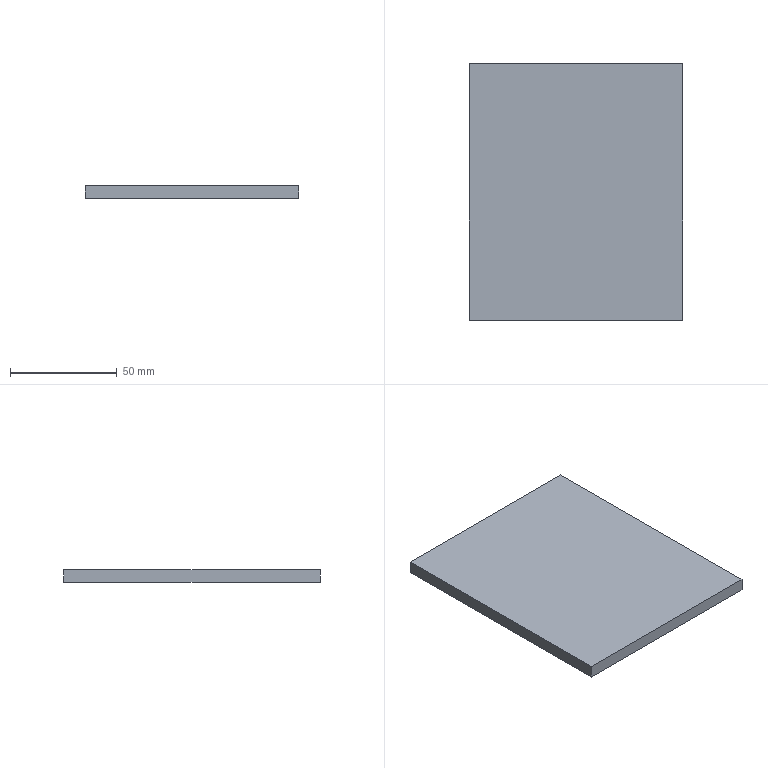Part | SolidWorks | features Extrusion 1 | 1 solid | 6 faces | box 100 x 120 x 6 mm | volume 72000 mm3 | plane 6
STEP:
#1=CARTESIAN_POINT('',(0.,0.,0.));
#2=VERTEX_POINT('',#1);
#3=CARTESIAN_POINT('',(100.,0.,0.));
#4=VERTEX_POINT('',#3);
#5=CARTESIAN_POINT('',(100.,0.,0.));
#6=DIRECTION('',(1.,0.,0.));
#7=VECTOR('',#6,1000.);
#8=LINE('',#5,#7);
#9=EDGE_CURVE('',#2,#4,#8,.T.);
#10=ORIENTED_EDGE('',*,*,#9,.T.);
#11=CARTESIAN_POINT('',(100.,0.,6.));
#12=VERTEX_POINT('',#11);
#13=CARTESIAN_POINT('',(100.,0.,6.));
#14=DIRECTION('',(0.,0.,-1.));
#15=VECTOR('',#14,1000.);
#16=LINE('',#13,#15);
#17=EDGE_CURVE('',#12,#4,#16,.T.);
#18=ORIENTED_EDGE('',*,*,#17,.F.);
#19=CARTESIAN_POINT('',(0.,0.,6.));
#20=VERTEX_POINT('',#19);
#21=CARTESIAN_POINT('',(100.,0.,6.));
#22=DIRECTION('',(1.,0.,0.));
#23=VECTOR('',#22,1000.);
#24=LINE('',#21,#23);
#25=EDGE_CURVE('',#20,#12,#24,.T.);
#26=ORIENTED_EDGE('',*,*,#25,.F.);
#27=CARTESIAN_POINT('',(0.,0.,6.));
#28=DIRECTION('',(0.,0.,-1.));
#29=VECTOR('',#28,1000.);
#30=LINE('',#27,#29);
#31=EDGE_CURVE('',#20,#2,#30,.T.);
#32=ORIENTED_EDGE('',*,*,#31,.T.);
#33=EDGE_LOOP('',(#10,#18,#26,#32));
#34=FACE_OUTER_BOUND('',#33,.T.);
#35=CARTESIAN_POINT('',(100.,0.,6.));
#36=DIRECTION('',(0.,1.,0.));
#37=DIRECTION('',(0.,0.,1.));
#38=AXIS2_PLACEMENT_3D('',#35,#36,#37);
#39=PLANE('',#38);
#40=ADVANCED_FACE('',(#34),#39,.F.);
#41=CARTESIAN_POINT('',(100.,120.,0.));
#42=VERTEX_POINT('',#41);
#43=CARTESIAN_POINT('',(100.,120.,0.));
#44=DIRECTION('',(0.,1.,0.));
#45=VECTOR('',#44,1000.);
#46=LINE('',#43,#45);
#47=EDGE_CURVE('',#4,#42,#46,.T.);
#48=ORIENTED_EDGE('',*,*,#47,.T.);
#49=CARTESIAN_POINT('',(100.,120.,6.));
#50=VERTEX_POINT('',#49);
#51=CARTESIAN_POINT('',(100.,120.,6.));
#52=DIRECTION('',(0.,0.,-1.));
#53=VECTOR('',#52,1000.);
#54=LINE('',#51,#53);
#55=EDGE_CURVE('',#50,#42,#54,.T.);
#56=ORIENTED_EDGE('',*,*,#55,.F.);
#57=CARTESIAN_POINT('',(100.,120.,6.));
#58=DIRECTION('',(0.,1.,0.));
#59=VECTOR('',#58,1000.);
#60=LINE('',#57,#59);
#61=EDGE_CURVE('',#12,#50,#60,.T.);
#62=ORIENTED_EDGE('',*,*,#61,.F.);
#63=ORIENTED_EDGE('',*,*,#17,.T.);
#64=EDGE_LOOP('',(#48,#56,#62,#63));
#65=FACE_OUTER_BOUND('',#64,.T.);
#66=CARTESIAN_POINT('',(100.,120.,6.));
#67=DIRECTION('',(-1.,0.,0.));
#68=DIRECTION('',(0.,0.,1.));
#69=AXIS2_PLACEMENT_3D('',#66,#67,#68);
#70=PLANE('',#69);
#71=ADVANCED_FACE('',(#65),#70,.F.);
#72=CARTESIAN_POINT('',(0.,120.,0.));
#73=VERTEX_POINT('',#72);
#74=CARTESIAN_POINT('',(0.,120.,0.));
#75=DIRECTION('',(-1.,0.,0.));
#76=VECTOR('',#75,1000.);
#77=LINE('',#74,#76);
#78=EDGE_CURVE('',#42,#73,#77,.T.);
#79=ORIENTED_EDGE('',*,*,#78,.T.);
#80=CARTESIAN_POINT('',(0.,120.,6.));
#81=VERTEX_POINT('',#80);
#82=CARTESIAN_POINT('',(0.,120.,6.));
#83=DIRECTION('',(0.,0.,-1.));
#84=VECTOR('',#83,1000.);
#85=LINE('',#82,#84);
#86=EDGE_CURVE('',#81,#73,#85,.T.);
#87=ORIENTED_EDGE('',*,*,#86,.F.);
#88=CARTESIAN_POINT('',(0.,120.,6.));
#89=DIRECTION('',(-1.,0.,0.));
#90=VECTOR('',#89,1000.);
#91=LINE('',#88,#90);
#92=EDGE_CURVE('',#50,#81,#91,.T.);
#93=ORIENTED_EDGE('',*,*,#92,.F.);
#94=ORIENTED_EDGE('',*,*,#55,.T.);
#95=EDGE_LOOP('',(#79,#87,#93,#94));
#96=FACE_OUTER_BOUND('',#95,.T.);
#97=CARTESIAN_POINT('',(0.,120.,6.));
#98=DIRECTION('',(0.,-1.,0.));
#99=DIRECTION('',(0.,0.,-1.));
#100=AXIS2_PLACEMENT_3D('',#97,#98,#99);
#101=PLANE('',#100);
#102=ADVANCED_FACE('',(#96),#101,.F.);
#103=CARTESIAN_POINT('',(0.,0.,0.));
#104=DIRECTION('',(0.,-1.,0.));
#105=VECTOR('',#104,1000.);
#106=LINE('',#103,#105);
#107=EDGE_CURVE('',#73,#2,#106,.T.);
#108=ORIENTED_EDGE('',*,*,#107,.T.);
#109=ORIENTED_EDGE('',*,*,#31,.F.);
#110=CARTESIAN_POINT('',(0.,0.,6.));
#111=DIRECTION('',(0.,-1.,0.));
#112=VECTOR('',#111,1000.);
#113=LINE('',#110,#112);
#114=EDGE_CURVE('',#81,#20,#113,.T.);
#115=ORIENTED_EDGE('',*,*,#114,.F.);
#116=ORIENTED_EDGE('',*,*,#86,.T.);
#117=EDGE_LOOP('',(#108,#109,#115,#116));
#118=FACE_OUTER_BOUND('',#117,.T.);
#119=CARTESIAN_POINT('',(0.,0.,6.));
#120=DIRECTION('',(1.,0.,0.));
#121=DIRECTION('',(0.,0.,-1.));
#122=AXIS2_PLACEMENT_3D('',#119,#120,#121);
#123=PLANE('',#122);
#124=ADVANCED_FACE('',(#118),#123,.F.);
#125=ORIENTED_EDGE('',*,*,#25,.T.);
#126=ORIENTED_EDGE('',*,*,#61,.T.);
#127=ORIENTED_EDGE('',*,*,#92,.T.);
#128=ORIENTED_EDGE('',*,*,#114,.T.);
#129=EDGE_LOOP('',(#125,#126,#127,#128));
#130=FACE_OUTER_BOUND('',#129,.T.);
#131=CARTESIAN_POINT('',(0.,0.,6.));
#132=DIRECTION('',(0.,0.,-1.));
#133=DIRECTION('',(-1.,0.,0.));
#134=AXIS2_PLACEMENT_3D('',#131,#132,#133);
#135=PLANE('',#134);
#136=ADVANCED_FACE('',(#130),#135,.F.);
#137=ORIENTED_EDGE('',*,*,#9,.F.);
#138=ORIENTED_EDGE('',*,*,#107,.F.);
#139=ORIENTED_EDGE('',*,*,#78,.F.);
#140=ORIENTED_EDGE('',*,*,#47,.F.);
#141=EDGE_LOOP('',(#137,#138,#139,#140));
#142=FACE_OUTER_BOUND('',#141,.T.);
#143=CARTESIAN_POINT('',(0.,0.,0.));
#144=DIRECTION('',(0.,0.,-1.));
#145=DIRECTION('',(-1.,0.,0.));
#146=AXIS2_PLACEMENT_3D('',#143,#144,#145);
#147=PLANE('',#146);
#148=ADVANCED_FACE('',(#142),#147,.T.);
#149=CLOSED_SHELL('',(#40,#71,#102,#124,#136,#148));
#150=MANIFOLD_SOLID_BREP('',#149);
#151=CARTESIAN_POINT('',(0.,0.,0.));
#152=DIRECTION('',(0.,0.,1.));
#153=DIRECTION('',(1.,0.,0.));
#154=AXIS2_PLACEMENT_3D('',#151,#152,#153);
#155=(LENGTH_UNIT()NAMED_UNIT(*)SI_UNIT(.MILLI.,.METRE.));
#156=UNCERTAINTY_MEASURE_WITH_UNIT(LENGTH_MEASURE(0.00001),#155,'','');
#157=(NAMED_UNIT(*)PLANE_ANGLE_UNIT()SI_UNIT($,.RADIAN.));
#158=(NAMED_UNIT(*)SI_UNIT($,.STERADIAN.)SOLID_ANGLE_UNIT());
#159=(GEOMETRIC_REPRESENTATION_CONTEXT(3)GLOBAL_UNCERTAINTY_ASSIGNED_CONTEXT((#156))GLOBAL_UNIT_ASSIGNED_CONTEXT((#155,#157,#158))REPRESENTATION_CONTEXT('',''));
#160=ADVANCED_BREP_SHAPE_REPRESENTATION('',(#150,#154),#159);